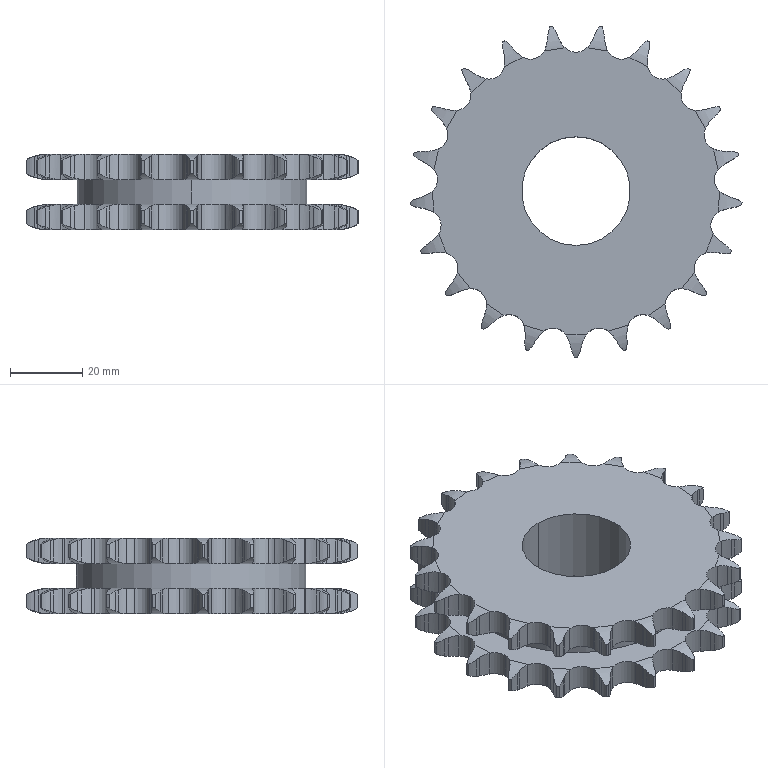Part | STEP file | 1 solid | 448 faces | box 91.67 x 91.415 x 20.973 mm | volume 80122 mm3 | cylinder 276 | plane 88 | spline 84 | commonest cylinder face diameters 14.045 x88 22.211 x88 8.595 x54 91.879 x42 30 x2 63.361 x2